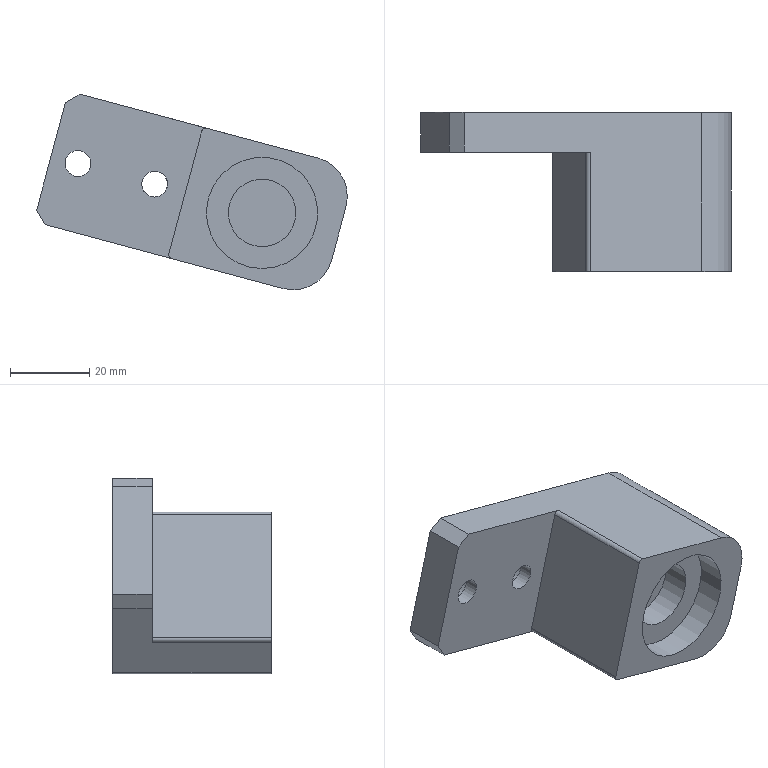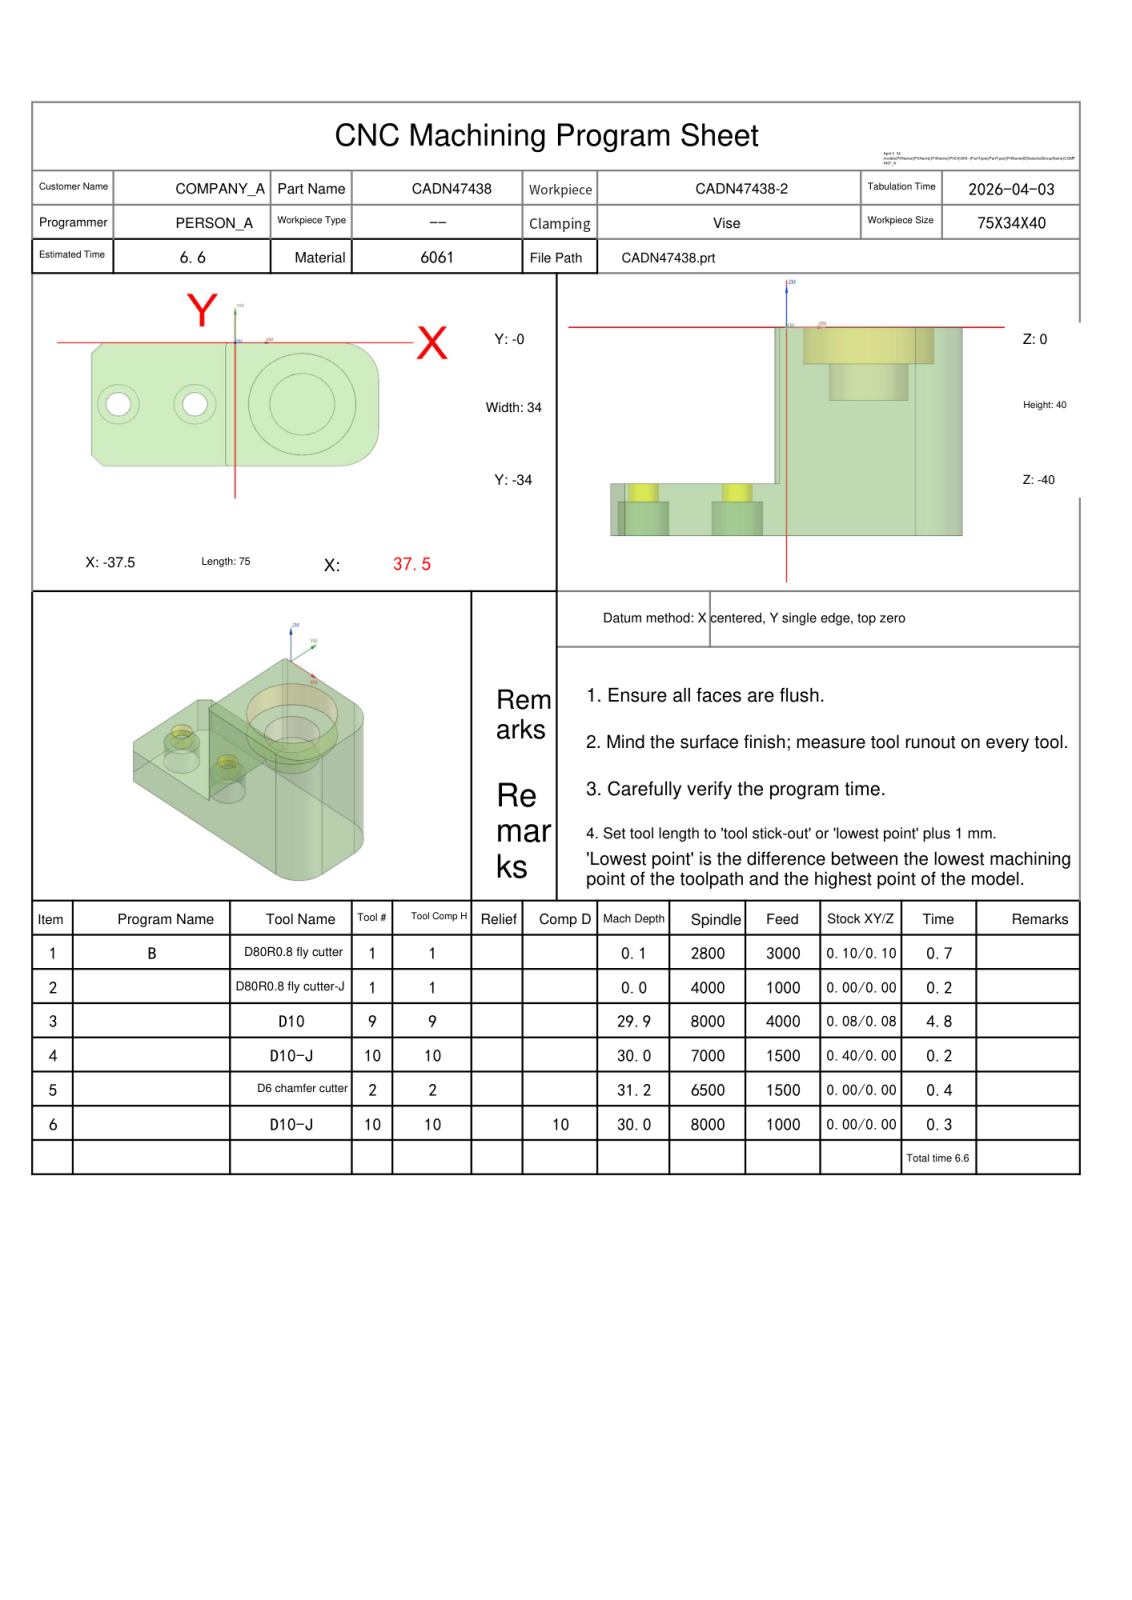NC program | NX | posted by the shop | part box 78.22 x 40 x 49.229 mm
Lines 1 to 108 of 2756:
%
O0001
(Machine time: 7.45 MIN)
(===Total Tool:4===)
(T1=D80R0.8 fly cutter D=80.  R=0.8  D-  H01 Z=0.    )
(T9=D10     D=10.  R=0.   D-  H09 Z=-29.9 )
(T10=D10-J  D=10.  R=0.   D-  H10 Z=-30.  )
(T2=D6 chamfer cutter   D=6.   R=0.   D-  H02 Z=-31.2 )
G80 G90 G17 G49 G40
G91 G28 Z0
M01
N1 T01 M06
(D80R0.8 fly cutter  D=80. R=0.8 H=01 ce=0.10 di=0.10)
G00 G90 G54 X89.597 Y-15.075 M03 S2800
G43 H01 Z20.
M08
Z6.011
G01 Z4.011 F3000.
X77.597 Y-15.323
X-77.597 Y-18.533
X-89.597 Y-18.781
Z6.011
G00 X89.597 Y-15.075
Z5.522
G01 Z3.522
X77.597 Y-15.323
X-77.597 Y-18.533
X-89.597 Y-18.781
Z5.522
G00 X89.597 Y-15.075
Z5.033
G01 Z3.033
X77.597 Y-15.323
X-77.597 Y-18.533
X-89.597 Y-18.781
Z5.033
G00 X89.597 Y-15.075
Z4.544
G01 Z2.544
X77.597 Y-15.323
X-77.597 Y-18.533
X-89.597 Y-18.781
Z4.544
G00 Z20.
X89.597 Y-15.075
Z4.056
G01 Z2.056
X77.597 Y-15.323
X-77.597 Y-18.533
X-89.597 Y-18.781
Z4.056
G00 Z20.
X89.597 Y-15.075
Z3.567
G01 Z1.567
X77.597 Y-15.323
X-77.597 Y-18.533
X-89.597 Y-18.781
Z3.567
G00 Z20.
X89.597 Y-15.075
Z3.078
G01 Z1.078
X77.597 Y-15.323
X-77.597 Y-18.533
X-89.597 Y-18.781
Z3.078
G00 Z20.
X89.597 Y-15.075
Z2.589
G01 Z.589
X77.597 Y-15.323
X-77.597 Y-18.533
X-89.597 Y-18.781
Z2.589
G00 Z20.
X89.597 Y-15.075
Z2.1
G01 Z.1
X77.597 Y-15.323
X-77.597 Y-18.533
X-89.597 Y-18.781
Z2.1
G00 Z20.
G91 G28 Z0.0
M05
M09
G91 G28 Z0.0
M01
N2 T01 M06
(D80R0.8 fly cutter-J  D=80. R=0.8 H=01 ce=0.00 di=0.00)
G00 G90 G54 X89.499 Y-15.079 M03 S4000
G43 H01 Z20.
M08
Z2.
G01 Z0.0 F1000.
X77.499 Y-15.327
X-77.499 Y-18.53
X-89.499 Y-18.778
Z2.
G00 Z20.
G91 G28 Z0.0
M05
M09
G91 G28 Z0.0
M01